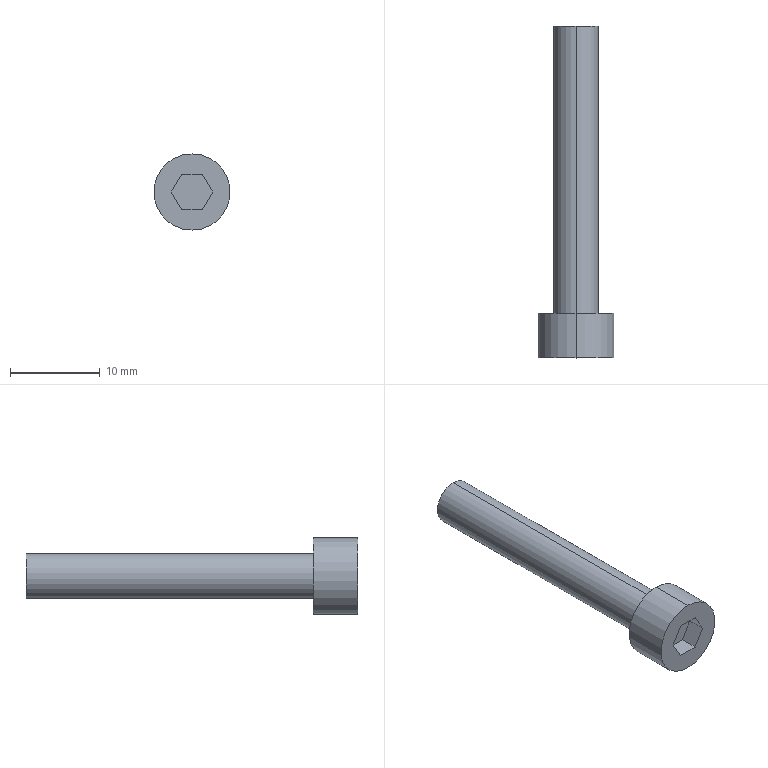Part | SolidWorks | features BaseBody 1 | 1 solid | 14 faces | box 8.5 x 37 x 8.5 mm | volume 884.331 mm3 | plane 10 | cylinder 4 | commonest cylinder face diameters 5 x2 8.5 x2
STEP:
#1=CARTESIAN_POINT('',(0.,37.,-2.5));
#2=VERTEX_POINT('',#1);
#3=CARTESIAN_POINT('',(0.,37.,2.5));
#4=VERTEX_POINT('',#3);
#5=CARTESIAN_POINT('',(0.,37.,0.));
#6=DIRECTION('',(0.,-1.,0.));
#7=DIRECTION('',(0.,0.,-1.));
#8=AXIS2_PLACEMENT_3D('',#5,#6,#7);
#9=CIRCLE('',#8,2.5);
#10=EDGE_CURVE('',#2,#4,#9,.T.);
#11=ORIENTED_EDGE('',*,*,#10,.T.);
#12=CARTESIAN_POINT('',(0.,5.,2.5));
#13=VERTEX_POINT('',#12);
#14=CARTESIAN_POINT('',(0.,37.,2.5));
#15=DIRECTION('',(0.,-1.,0.));
#16=VECTOR('',#15,1000.);
#17=LINE('',#14,#16);
#18=EDGE_CURVE('',#4,#13,#17,.T.);
#19=ORIENTED_EDGE('',*,*,#18,.T.);
#20=CARTESIAN_POINT('',(0.,5.,-2.5));
#21=VERTEX_POINT('',#20);
#22=CARTESIAN_POINT('',(0.,5.,0.));
#23=DIRECTION('',(0.,1.,0.));
#24=DIRECTION('',(0.,0.,-1.));
#25=AXIS2_PLACEMENT_3D('',#22,#23,#24);
#26=CIRCLE('',#25,2.5);
#27=EDGE_CURVE('',#13,#21,#26,.T.);
#28=ORIENTED_EDGE('',*,*,#27,.T.);
#29=CARTESIAN_POINT('',(0.,37.,-2.5));
#30=DIRECTION('',(0.,-1.,0.));
#31=VECTOR('',#30,1000.);
#32=LINE('',#29,#31);
#33=EDGE_CURVE('',#2,#21,#32,.T.);
#34=ORIENTED_EDGE('',*,*,#33,.F.);
#35=EDGE_LOOP('',(#11,#19,#28,#34));
#36=FACE_OUTER_BOUND('',#35,.T.);
#37=CARTESIAN_POINT('',(0.,37.,0.));
#38=DIRECTION('',(0.,-1.,0.));
#39=DIRECTION('',(0.,0.,-1.));
#40=AXIS2_PLACEMENT_3D('',#37,#38,#39);
#41=CYLINDRICAL_SURFACE('',#40,2.5);
#42=ADVANCED_FACE('',(#36),#41,.T.);
#43=CARTESIAN_POINT('',(0.,5.,4.25));
#44=VERTEX_POINT('',#43);
#45=CARTESIAN_POINT('',(0.,5.,-4.25));
#46=VERTEX_POINT('',#45);
#47=CARTESIAN_POINT('',(0.,5.,0.));
#48=DIRECTION('',(0.,1.,0.));
#49=DIRECTION('',(0.,0.,-1.));
#50=AXIS2_PLACEMENT_3D('',#47,#48,#49);
#51=CIRCLE('',#50,4.25);
#52=EDGE_CURVE('',#44,#46,#51,.T.);
#53=ORIENTED_EDGE('',*,*,#52,.F.);
#54=CARTESIAN_POINT('',(0.,0.,4.25));
#55=VERTEX_POINT('',#54);
#56=CARTESIAN_POINT('',(0.,5.,4.25));
#57=DIRECTION('',(0.,-1.,0.));
#58=VECTOR('',#57,1000.);
#59=LINE('',#56,#58);
#60=EDGE_CURVE('',#44,#55,#59,.T.);
#61=ORIENTED_EDGE('',*,*,#60,.T.);
#62=CARTESIAN_POINT('',(0.,0.,-4.25));
#63=VERTEX_POINT('',#62);
#64=CARTESIAN_POINT('',(0.,0.,0.));
#65=DIRECTION('',(0.,1.,0.));
#66=DIRECTION('',(0.,0.,-1.));
#67=AXIS2_PLACEMENT_3D('',#64,#65,#66);
#68=CIRCLE('',#67,4.25);
#69=EDGE_CURVE('',#55,#63,#68,.T.);
#70=ORIENTED_EDGE('',*,*,#69,.T.);
#71=CARTESIAN_POINT('',(0.,5.,-4.25));
#72=DIRECTION('',(0.,-1.,0.));
#73=VECTOR('',#72,1000.);
#74=LINE('',#71,#73);
#75=EDGE_CURVE('',#46,#63,#74,.T.);
#76=ORIENTED_EDGE('',*,*,#75,.F.);
#77=EDGE_LOOP('',(#53,#61,#70,#76));
#78=FACE_OUTER_BOUND('',#77,.T.);
#79=CARTESIAN_POINT('',(0.,5.,0.));
#80=DIRECTION('',(0.,-1.,0.));
#81=DIRECTION('',(0.,0.,-1.));
#82=AXIS2_PLACEMENT_3D('',#79,#80,#81);
#83=CYLINDRICAL_SURFACE('',#82,4.25);
#84=ADVANCED_FACE('',(#78),#83,.T.);
#85=ORIENTED_EDGE('',*,*,#18,.F.);
#86=CARTESIAN_POINT('',(0.,37.,0.));
#87=DIRECTION('',(0.,-1.,0.));
#88=DIRECTION('',(0.,0.,-1.));
#89=AXIS2_PLACEMENT_3D('',#86,#87,#88);
#90=CIRCLE('',#89,2.5);
#91=EDGE_CURVE('',#4,#2,#90,.T.);
#92=ORIENTED_EDGE('',*,*,#91,.T.);
#93=ORIENTED_EDGE('',*,*,#33,.T.);
#94=CARTESIAN_POINT('',(0.,5.,0.));
#95=DIRECTION('',(0.,1.,0.));
#96=DIRECTION('',(0.,0.,-1.));
#97=AXIS2_PLACEMENT_3D('',#94,#95,#96);
#98=CIRCLE('',#97,2.5);
#99=EDGE_CURVE('',#21,#13,#98,.T.);
#100=ORIENTED_EDGE('',*,*,#99,.T.);
#101=EDGE_LOOP('',(#85,#92,#93,#100));
#102=FACE_OUTER_BOUND('',#101,.T.);
#103=CARTESIAN_POINT('',(0.,37.,0.));
#104=DIRECTION('',(0.,-1.,0.));
#105=DIRECTION('',(0.,0.,-1.));
#106=AXIS2_PLACEMENT_3D('',#103,#104,#105);
#107=CYLINDRICAL_SURFACE('',#106,2.5);
#108=ADVANCED_FACE('',(#102),#107,.T.);
#109=CARTESIAN_POINT('',(0.,5.,0.));
#110=DIRECTION('',(0.,1.,0.));
#111=DIRECTION('',(0.,0.,-1.));
#112=AXIS2_PLACEMENT_3D('',#109,#110,#111);
#113=CIRCLE('',#112,4.25);
#114=EDGE_CURVE('',#46,#44,#113,.T.);
#115=ORIENTED_EDGE('',*,*,#114,.T.);
#116=ORIENTED_EDGE('',*,*,#52,.T.);
#117=EDGE_LOOP('',(#115,#116));
#118=FACE_OUTER_BOUND('',#117,.T.);
#119=ORIENTED_EDGE('',*,*,#99,.F.);
#120=ORIENTED_EDGE('',*,*,#27,.F.);
#121=EDGE_LOOP('',(#119,#120));
#122=FACE_BOUND('',#121,.T.);
#123=CARTESIAN_POINT('',(0.,5.,0.));
#124=DIRECTION('',(0.,1.,0.));
#125=DIRECTION('',(0.,0.,1.));
#126=AXIS2_PLACEMENT_3D('',#123,#124,#125);
#127=PLANE('',#126);
#128=ADVANCED_FACE('',(#118,#122),#127,.T.);
#129=ORIENTED_EDGE('',*,*,#10,.F.);
#130=ORIENTED_EDGE('',*,*,#91,.F.);
#131=EDGE_LOOP('',(#129,#130));
#132=FACE_OUTER_BOUND('',#131,.T.);
#133=CARTESIAN_POINT('',(0.,37.,0.));
#134=DIRECTION('',(0.,1.,0.));
#135=DIRECTION('',(0.,0.,1.));
#136=AXIS2_PLACEMENT_3D('',#133,#134,#135);
#137=PLANE('',#136);
#138=ADVANCED_FACE('',(#132),#137,.T.);
#139=ORIENTED_EDGE('',*,*,#60,.F.);
#140=ORIENTED_EDGE('',*,*,#114,.F.);
#141=ORIENTED_EDGE('',*,*,#75,.T.);
#142=CARTESIAN_POINT('',(0.,0.,0.));
#143=DIRECTION('',(0.,1.,0.));
#144=DIRECTION('',(0.,0.,-1.));
#145=AXIS2_PLACEMENT_3D('',#142,#143,#144);
#146=CIRCLE('',#145,4.25);
#147=EDGE_CURVE('',#63,#55,#146,.T.);
#148=ORIENTED_EDGE('',*,*,#147,.T.);
#149=EDGE_LOOP('',(#139,#140,#141,#148));
#150=FACE_OUTER_BOUND('',#149,.T.);
#151=CARTESIAN_POINT('',(0.,5.,0.));
#152=DIRECTION('',(0.,-1.,0.));
#153=DIRECTION('',(0.,0.,-1.));
#154=AXIS2_PLACEMENT_3D('',#151,#152,#153);
#155=CYLINDRICAL_SURFACE('',#154,4.25);
#156=ADVANCED_FACE('',(#150),#155,.T.);
#157=ORIENTED_EDGE('',*,*,#147,.F.);
#158=ORIENTED_EDGE('',*,*,#69,.F.);
#159=EDGE_LOOP('',(#157,#158));
#160=FACE_OUTER_BOUND('',#159,.T.);
#161=CARTESIAN_POINT('',(1.155,0.,-2.));
#162=VERTEX_POINT('',#161);
#163=CARTESIAN_POINT('',(2.309,0.,0.));
#164=VERTEX_POINT('',#163);
#165=CARTESIAN_POINT('',(1.155,0.,-2.));
#166=DIRECTION('',(0.5,0.,0.866));
#167=VECTOR('',#166,1000.);
#168=LINE('',#165,#167);
#169=EDGE_CURVE('',#162,#164,#168,.T.);
#170=ORIENTED_EDGE('',*,*,#169,.F.);
#171=CARTESIAN_POINT('',(-1.155,0.,-2.));
#172=VERTEX_POINT('',#171);
#173=CARTESIAN_POINT('',(0.,0.,-2.));
#174=DIRECTION('',(1.,0.,0.));
#175=VECTOR('',#174,1000.);
#176=LINE('',#173,#175);
#177=EDGE_CURVE('',#172,#162,#176,.T.);
#178=ORIENTED_EDGE('',*,*,#177,.F.);
#179=CARTESIAN_POINT('',(-2.309,0.,0.));
#180=VERTEX_POINT('',#179);
#181=CARTESIAN_POINT('',(-2.309,0.,0.));
#182=DIRECTION('',(0.5,0.,-0.866));
#183=VECTOR('',#182,1000.);
#184=LINE('',#181,#183);
#185=EDGE_CURVE('',#180,#172,#184,.T.);
#186=ORIENTED_EDGE('',*,*,#185,.F.);
#187=CARTESIAN_POINT('',(-1.155,0.,2.));
#188=VERTEX_POINT('',#187);
#189=CARTESIAN_POINT('',(-1.155,0.,2.));
#190=DIRECTION('',(-0.5,0.,-0.866));
#191=VECTOR('',#190,1000.);
#192=LINE('',#189,#191);
#193=EDGE_CURVE('',#188,#180,#192,.T.);
#194=ORIENTED_EDGE('',*,*,#193,.F.);
#195=CARTESIAN_POINT('',(1.155,0.,2.));
#196=VERTEX_POINT('',#195);
#197=CARTESIAN_POINT('',(0.,0.,2.));
#198=DIRECTION('',(-1.,0.,0.));
#199=VECTOR('',#198,1000.);
#200=LINE('',#197,#199);
#201=EDGE_CURVE('',#196,#188,#200,.T.);
#202=ORIENTED_EDGE('',*,*,#201,.F.);
#203=CARTESIAN_POINT('',(2.309,0.,0.));
#204=DIRECTION('',(-0.5,0.,0.866));
#205=VECTOR('',#204,1000.);
#206=LINE('',#203,#205);
#207=EDGE_CURVE('',#164,#196,#206,.T.);
#208=ORIENTED_EDGE('',*,*,#207,.F.);
#209=EDGE_LOOP('',(#170,#178,#186,#194,#202,#208));
#210=FACE_BOUND('',#209,.T.);
#211=CARTESIAN_POINT('',(0.,0.,0.));
#212=DIRECTION('',(0.,1.,0.));
#213=DIRECTION('',(0.,0.,1.));
#214=AXIS2_PLACEMENT_3D('',#211,#212,#213);
#215=PLANE('',#214);
#216=ADVANCED_FACE('',(#160,#210),#215,.F.);
#217=CARTESIAN_POINT('',(1.155,2.,2.));
#218=VERTEX_POINT('',#217);
#219=CARTESIAN_POINT('',(1.155,2.,2.));
#220=DIRECTION('',(0.,-1.,0.));
#221=VECTOR('',#220,1000.);
#222=LINE('',#219,#221);
#223=EDGE_CURVE('',#218,#196,#222,.T.);
#224=ORIENTED_EDGE('',*,*,#223,.F.);
#225=CARTESIAN_POINT('',(2.309,2.,0.));
#226=VERTEX_POINT('',#225);
#227=CARTESIAN_POINT('',(2.309,2.,0.));
#228=DIRECTION('',(-0.5,0.,0.866));
#229=VECTOR('',#228,1000.);
#230=LINE('',#227,#229);
#231=EDGE_CURVE('',#226,#218,#230,.T.);
#232=ORIENTED_EDGE('',*,*,#231,.F.);
#233=CARTESIAN_POINT('',(2.309,2.,0.));
#234=DIRECTION('',(0.,1.,0.));
#235=VECTOR('',#234,1000.);
#236=LINE('',#233,#235);
#237=EDGE_CURVE('',#164,#226,#236,.T.);
#238=ORIENTED_EDGE('',*,*,#237,.F.);
#239=ORIENTED_EDGE('',*,*,#207,.T.);
#240=EDGE_LOOP('',(#224,#232,#238,#239));
#241=FACE_OUTER_BOUND('',#240,.T.);
#242=CARTESIAN_POINT('',(2.309,2.,0.));
#243=DIRECTION('',(0.866,0.,0.5));
#244=DIRECTION('',(0.5,0.,-0.866));
#245=AXIS2_PLACEMENT_3D('',#242,#243,#244);
#246=PLANE('',#245);
#247=ADVANCED_FACE('',(#241),#246,.F.);
#248=ORIENTED_EDGE('',*,*,#237,.T.);
#249=CARTESIAN_POINT('',(1.155,2.,-2.));
#250=VERTEX_POINT('',#249);
#251=CARTESIAN_POINT('',(1.155,2.,-2.));
#252=DIRECTION('',(0.5,0.,0.866));
#253=VECTOR('',#252,1000.);
#254=LINE('',#251,#253);
#255=EDGE_CURVE('',#250,#226,#254,.T.);
#256=ORIENTED_EDGE('',*,*,#255,.F.);
#257=CARTESIAN_POINT('',(1.155,2.,-2.));
#258=DIRECTION('',(0.,1.,0.));
#259=VECTOR('',#258,1000.);
#260=LINE('',#257,#259);
#261=EDGE_CURVE('',#162,#250,#260,.T.);
#262=ORIENTED_EDGE('',*,*,#261,.F.);
#263=ORIENTED_EDGE('',*,*,#169,.T.);
#264=EDGE_LOOP('',(#248,#256,#262,#263));
#265=FACE_OUTER_BOUND('',#264,.T.);
#266=CARTESIAN_POINT('',(1.155,2.,-2.));
#267=DIRECTION('',(0.866,0.,-0.5));
#268=DIRECTION('',(-0.5,0.,-0.866));
#269=AXIS2_PLACEMENT_3D('',#266,#267,#268);
#270=PLANE('',#269);
#271=ADVANCED_FACE('',(#265),#270,.F.);
#272=ORIENTED_EDGE('',*,*,#261,.T.);
#273=CARTESIAN_POINT('',(-1.155,2.,-2.));
#274=VERTEX_POINT('',#273);
#275=CARTESIAN_POINT('',(-1.155,2.,-2.));
#276=DIRECTION('',(1.,0.,0.));
#277=VECTOR('',#276,1000.);
#278=LINE('',#275,#277);
#279=EDGE_CURVE('',#274,#250,#278,.T.);
#280=ORIENTED_EDGE('',*,*,#279,.F.);
#281=CARTESIAN_POINT('',(-1.155,2.,-2.));
#282=DIRECTION('',(0.,1.,0.));
#283=VECTOR('',#282,1000.);
#284=LINE('',#281,#283);
#285=EDGE_CURVE('',#172,#274,#284,.T.);
#286=ORIENTED_EDGE('',*,*,#285,.F.);
#287=ORIENTED_EDGE('',*,*,#177,.T.);
#288=EDGE_LOOP('',(#272,#280,#286,#287));
#289=FACE_OUTER_BOUND('',#288,.T.);
#290=CARTESIAN_POINT('',(-1.155,2.,-2.));
#291=DIRECTION('',(0.,0.,-1.));
#292=DIRECTION('',(-1.,0.,0.));
#293=AXIS2_PLACEMENT_3D('',#290,#291,#292);
#294=PLANE('',#293);
#295=ADVANCED_FACE('',(#289),#294,.F.);
#296=ORIENTED_EDGE('',*,*,#285,.T.);
#297=CARTESIAN_POINT('',(-2.309,2.,0.));
#298=VERTEX_POINT('',#297);
#299=CARTESIAN_POINT('',(-2.309,2.,0.));
#300=DIRECTION('',(0.5,0.,-0.866));
#301=VECTOR('',#300,1000.);
#302=LINE('',#299,#301);
#303=EDGE_CURVE('',#298,#274,#302,.T.);
#304=ORIENTED_EDGE('',*,*,#303,.F.);
#305=CARTESIAN_POINT('',(-2.309,2.,0.));
#306=DIRECTION('',(0.,1.,0.));
#307=VECTOR('',#306,1000.);
#308=LINE('',#305,#307);
#309=EDGE_CURVE('',#180,#298,#308,.T.);
#310=ORIENTED_EDGE('',*,*,#309,.F.);
#311=ORIENTED_EDGE('',*,*,#185,.T.);
#312=EDGE_LOOP('',(#296,#304,#310,#311));
#313=FACE_OUTER_BOUND('',#312,.T.);
#314=CARTESIAN_POINT('',(-2.309,2.,0.));
#315=DIRECTION('',(-0.866,0.,-0.5));
#316=DIRECTION('',(-0.5,0.,0.866));
#317=AXIS2_PLACEMENT_3D('',#314,#315,#316);
#318=PLANE('',#317);
#319=ADVANCED_FACE('',(#313),#318,.F.);
#320=ORIENTED_EDGE('',*,*,#309,.T.);
#321=CARTESIAN_POINT('',(-1.155,2.,2.));
#322=VERTEX_POINT('',#321);
#323=CARTESIAN_POINT('',(-1.155,2.,2.));
#324=DIRECTION('',(-0.5,0.,-0.866));
#325=VECTOR('',#324,1000.);
#326=LINE('',#323,#325);
#327=EDGE_CURVE('',#322,#298,#326,.T.);
#328=ORIENTED_EDGE('',*,*,#327,.F.);
#329=CARTESIAN_POINT('',(-1.155,2.,2.));
#330=DIRECTION('',(0.,1.,0.));
#331=VECTOR('',#330,1000.);
#332=LINE('',#329,#331);
#333=EDGE_CURVE('',#188,#322,#332,.T.);
#334=ORIENTED_EDGE('',*,*,#333,.F.);
#335=ORIENTED_EDGE('',*,*,#193,.T.);
#336=EDGE_LOOP('',(#320,#328,#334,#335));
#337=FACE_OUTER_BOUND('',#336,.T.);
#338=CARTESIAN_POINT('',(-1.155,2.,2.));
#339=DIRECTION('',(-0.866,0.,0.5));
#340=DIRECTION('',(0.5,0.,0.866));
#341=AXIS2_PLACEMENT_3D('',#338,#339,#340);
#342=PLANE('',#341);
#343=ADVANCED_FACE('',(#337),#342,.F.);
#344=ORIENTED_EDGE('',*,*,#333,.T.);
#345=CARTESIAN_POINT('',(1.155,2.,2.));
#346=DIRECTION('',(-1.,0.,0.));
#347=VECTOR('',#346,1000.);
#348=LINE('',#345,#347);
#349=EDGE_CURVE('',#218,#322,#348,.T.);
#350=ORIENTED_EDGE('',*,*,#349,.F.);
#351=ORIENTED_EDGE('',*,*,#223,.T.);
#352=ORIENTED_EDGE('',*,*,#201,.T.);
#353=EDGE_LOOP('',(#344,#350,#351,#352));
#354=FACE_OUTER_BOUND('',#353,.T.);
#355=CARTESIAN_POINT('',(1.155,2.,2.));
#356=DIRECTION('',(0.,0.,1.));
#357=DIRECTION('',(1.,0.,0.));
#358=AXIS2_PLACEMENT_3D('',#355,#356,#357);
#359=PLANE('',#358);
#360=ADVANCED_FACE('',(#354),#359,.F.);
#361=ORIENTED_EDGE('',*,*,#303,.T.);
#362=ORIENTED_EDGE('',*,*,#279,.T.);
#363=ORIENTED_EDGE('',*,*,#255,.T.);
#364=ORIENTED_EDGE('',*,*,#231,.T.);
#365=ORIENTED_EDGE('',*,*,#349,.T.);
#366=ORIENTED_EDGE('',*,*,#327,.T.);
#367=EDGE_LOOP('',(#361,#362,#363,#364,#365,#366));
#368=FACE_OUTER_BOUND('',#367,.T.);
#369=CARTESIAN_POINT('',(0.,2.,0.));
#370=DIRECTION('',(0.,-1.,0.));
#371=DIRECTION('',(0.,0.,-1.));
#372=AXIS2_PLACEMENT_3D('',#369,#370,#371);
#373=PLANE('',#372);
#374=ADVANCED_FACE('',(#368),#373,.T.);
#375=CLOSED_SHELL('',(#42,#84,#108,#128,#138,#156,#216,#247,#271,#295,#319,#343,#360,#374));
#376=MANIFOLD_SOLID_BREP('',#375);
#377=CARTESIAN_POINT('',(0.,0.,0.));
#378=DIRECTION('',(0.,0.,1.));
#379=DIRECTION('',(1.,0.,0.));
#380=AXIS2_PLACEMENT_3D('',#377,#378,#379);
#381=(LENGTH_UNIT()NAMED_UNIT(*)SI_UNIT(.MILLI.,.METRE.));
#382=UNCERTAINTY_MEASURE_WITH_UNIT(LENGTH_MEASURE(0.00001),#381,'','');
#383=(NAMED_UNIT(*)PLANE_ANGLE_UNIT()SI_UNIT($,.RADIAN.));
#384=(NAMED_UNIT(*)SI_UNIT($,.STERADIAN.)SOLID_ANGLE_UNIT());
#385=(GEOMETRIC_REPRESENTATION_CONTEXT(3)GLOBAL_UNCERTAINTY_ASSIGNED_CONTEXT((#382))GLOBAL_UNIT_ASSIGNED_CONTEXT((#381,#383,#384))REPRESENTATION_CONTEXT('',''));
#386=ADVANCED_BREP_SHAPE_REPRESENTATION('',(#376,#380),#385);